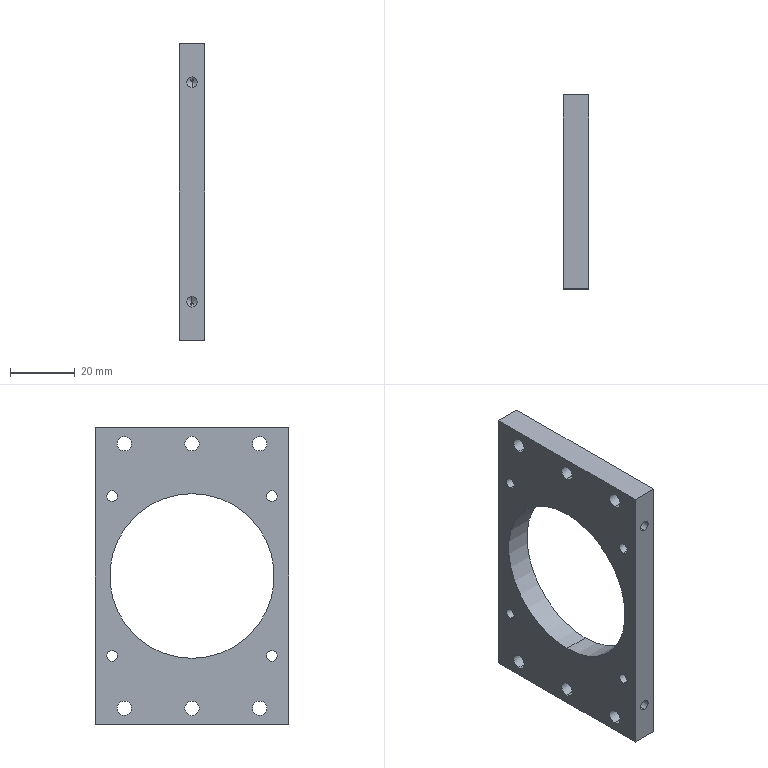Part | SolidWorks | features HoleWzd 3, Extrusion 1, ICE 1 | 1 solid | 54 faces | box 8 x 60 x 92 mm | volume 25695 mm3 | cylinder 38 | plane 12 | cone 4 | commonest cylinder face diameters 3.3 x12 4.5 x12 8 x12 51 x2